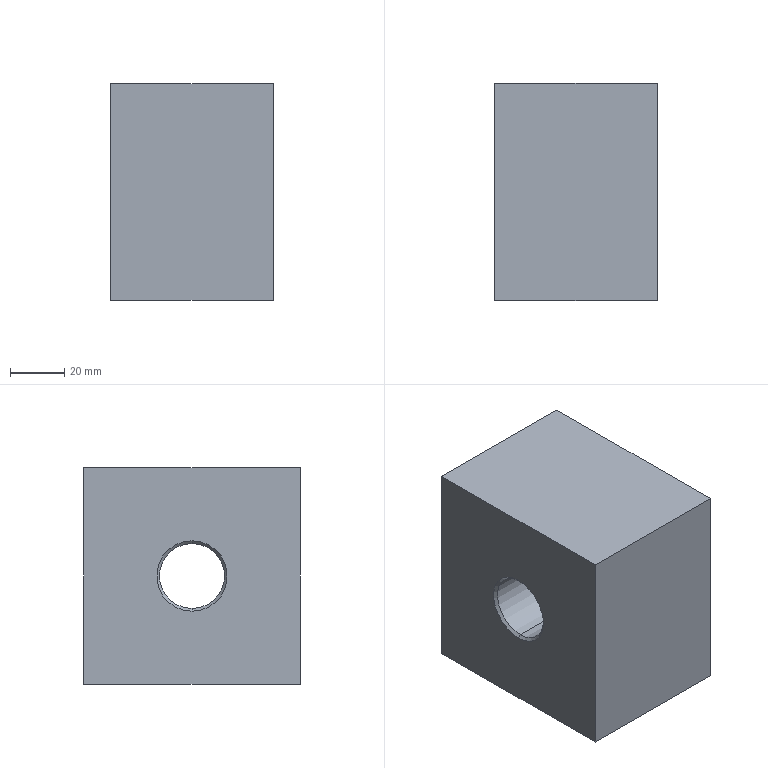Part | SolidWorks | features BaseBody 1 | 1 solid | 28 faces | box 60 x 80 x 80 mm | volume 348755 mm3 | cone 12 | cylinder 10 | plane 6 | commonest cylinder face diameters 8.5 x8 24 x2
STEP:
#1=CARTESIAN_POINT('',(29.,0.,12.));
#2=VERTEX_POINT('',#1);
#3=CARTESIAN_POINT('',(29.,0.,-12.));
#4=VERTEX_POINT('',#3);
#5=CARTESIAN_POINT('',(29.,0.,0.));
#6=DIRECTION('',(1.,0.,0.));
#7=DIRECTION('',(0.,0.,-1.));
#8=AXIS2_PLACEMENT_3D('',#5,#6,#7);
#9=CIRCLE('',#8,12.);
#10=EDGE_CURVE('',#2,#4,#9,.T.);
#11=ORIENTED_EDGE('',*,*,#10,.F.);
#12=CARTESIAN_POINT('',(30.,0.,13.));
#13=VERTEX_POINT('',#12);
#14=CARTESIAN_POINT('',(29.,0.,12.));
#15=DIRECTION('',(0.7071,0.,0.7071));
#16=VECTOR('',#15,1000.);
#17=LINE('',#14,#16);
#18=EDGE_CURVE('',#2,#13,#17,.T.);
#19=ORIENTED_EDGE('',*,*,#18,.T.);
#20=CARTESIAN_POINT('',(30.,0.,-13.));
#21=VERTEX_POINT('',#20);
#22=CARTESIAN_POINT('',(30.,0.,0.));
#23=DIRECTION('',(-1.,0.,0.));
#24=DIRECTION('',(0.,0.,-1.));
#25=AXIS2_PLACEMENT_3D('',#22,#23,#24);
#26=CIRCLE('',#25,13.);
#27=EDGE_CURVE('',#21,#13,#26,.T.);
#28=ORIENTED_EDGE('',*,*,#27,.F.);
#29=CARTESIAN_POINT('',(29.,0.,-12.));
#30=DIRECTION('',(0.7071,0.,-0.7071));
#31=VECTOR('',#30,1000.);
#32=LINE('',#29,#31);
#33=EDGE_CURVE('',#4,#21,#32,.T.);
#34=ORIENTED_EDGE('',*,*,#33,.F.);
#35=EDGE_LOOP('',(#11,#19,#28,#34));
#36=FACE_OUTER_BOUND('',#35,.T.);
#37=CARTESIAN_POINT('',(29.,0.,0.));
#38=DIRECTION('',(1.,0.,0.));
#39=DIRECTION('',(0.,0.,-1.));
#40=AXIS2_PLACEMENT_3D('',#37,#38,#39);
#41=CONICAL_SURFACE('',#40,12.,0.7854);
#42=ADVANCED_FACE('',(#36),#41,.F.);
#43=CARTESIAN_POINT('',(-29.,0.,-12.));
#44=VERTEX_POINT('',#43);
#45=CARTESIAN_POINT('',(-29.,0.,12.));
#46=VERTEX_POINT('',#45);
#47=CARTESIAN_POINT('',(-29.,0.,0.));
#48=DIRECTION('',(-1.,0.,0.));
#49=DIRECTION('',(0.,0.,-1.));
#50=AXIS2_PLACEMENT_3D('',#47,#48,#49);
#51=CIRCLE('',#50,12.);
#52=EDGE_CURVE('',#44,#46,#51,.T.);
#53=ORIENTED_EDGE('',*,*,#52,.F.);
#54=CARTESIAN_POINT('',(-30.,0.,-13.));
#55=VERTEX_POINT('',#54);
#56=CARTESIAN_POINT('',(-30.,0.,-13.));
#57=DIRECTION('',(-0.7071,0.,-0.7071));
#58=VECTOR('',#57,1000.);
#59=LINE('',#56,#58);
#60=EDGE_CURVE('',#44,#55,#59,.T.);
#61=ORIENTED_EDGE('',*,*,#60,.T.);
#62=CARTESIAN_POINT('',(-30.,0.,13.));
#63=VERTEX_POINT('',#62);
#64=CARTESIAN_POINT('',(-30.,0.,0.));
#65=DIRECTION('',(1.,0.,0.));
#66=DIRECTION('',(0.,0.,-1.));
#67=AXIS2_PLACEMENT_3D('',#64,#65,#66);
#68=CIRCLE('',#67,13.);
#69=EDGE_CURVE('',#63,#55,#68,.T.);
#70=ORIENTED_EDGE('',*,*,#69,.F.);
#71=CARTESIAN_POINT('',(-30.,0.,13.));
#72=DIRECTION('',(-0.7071,0.,0.7071));
#73=VECTOR('',#72,1000.);
#74=LINE('',#71,#73);
#75=EDGE_CURVE('',#46,#63,#74,.T.);
#76=ORIENTED_EDGE('',*,*,#75,.F.);
#77=EDGE_LOOP('',(#53,#61,#70,#76));
#78=FACE_OUTER_BOUND('',#77,.T.);
#79=CARTESIAN_POINT('',(-30.,0.,0.));
#80=DIRECTION('',(-1.,0.,0.));
#81=DIRECTION('',(0.,0.,1.));
#82=AXIS2_PLACEMENT_3D('',#79,#80,#81);
#83=CONICAL_SURFACE('',#82,13.,0.7854);
#84=ADVANCED_FACE('',(#78),#83,.F.);
#85=CARTESIAN_POINT('',(-15.,5.5,20.75));
#86=VERTEX_POINT('',#85);
#87=CARTESIAN_POINT('',(-15.,5.5,29.25));
#88=VERTEX_POINT('',#87);
#89=CARTESIAN_POINT('',(-15.,5.5,25.));
#90=DIRECTION('',(0.,1.,0.));
#91=DIRECTION('',(0.,0.,1.));
#92=AXIS2_PLACEMENT_3D('',#89,#90,#91);
#93=CIRCLE('',#92,4.25);
#94=EDGE_CURVE('',#86,#88,#93,.T.);
#95=ORIENTED_EDGE('',*,*,#94,.F.);
#96=CARTESIAN_POINT('',(-15.,40.,20.75));
#97=VERTEX_POINT('',#96);
#98=CARTESIAN_POINT('',(-15.,40.,20.75));
#99=DIRECTION('',(0.,1.,0.));
#100=VECTOR('',#99,1000.);
#101=LINE('',#98,#100);
#102=EDGE_CURVE('',#86,#97,#101,.T.);
#103=ORIENTED_EDGE('',*,*,#102,.T.);
#104=CARTESIAN_POINT('',(-15.,40.,29.25));
#105=VERTEX_POINT('',#104);
#106=CARTESIAN_POINT('',(-15.,40.,25.));
#107=DIRECTION('',(0.,1.,0.));
#108=DIRECTION('',(0.,0.,1.));
#109=AXIS2_PLACEMENT_3D('',#106,#107,#108);
#110=CIRCLE('',#109,4.25);
#111=EDGE_CURVE('',#97,#105,#110,.T.);
#112=ORIENTED_EDGE('',*,*,#111,.T.);
#113=CARTESIAN_POINT('',(-15.,40.,29.25));
#114=DIRECTION('',(0.,1.,0.));
#115=VECTOR('',#114,1000.);
#116=LINE('',#113,#115);
#117=EDGE_CURVE('',#88,#105,#116,.T.);
#118=ORIENTED_EDGE('',*,*,#117,.F.);
#119=EDGE_LOOP('',(#95,#103,#112,#118));
#120=FACE_OUTER_BOUND('',#119,.T.);
#121=CARTESIAN_POINT('',(-15.,40.,25.));
#122=DIRECTION('',(0.,1.,0.));
#123=DIRECTION('',(0.,0.,1.));
#124=AXIS2_PLACEMENT_3D('',#121,#122,#123);
#125=CYLINDRICAL_SURFACE('',#124,4.25);
#126=ADVANCED_FACE('',(#120),#125,.F.);
#127=CARTESIAN_POINT('',(-15.,2.946,25.));
#128=VERTEX_POINT('',#127);
#129=CARTESIAN_POINT('',(-15.,5.5,29.25));
#130=DIRECTION('',(0.,0.515,0.8572));
#131=VECTOR('',#130,1000.);
#132=LINE('',#129,#131);
#133=EDGE_CURVE('',#128,#88,#132,.T.);
#134=ORIENTED_EDGE('',*,*,#133,.F.);
#135=CARTESIAN_POINT('',(-15.,5.5,20.75));
#136=DIRECTION('',(0.,0.515,-0.8572));
#137=VECTOR('',#136,1000.);
#138=LINE('',#135,#137);
#139=EDGE_CURVE('',#128,#86,#138,.T.);
#140=ORIENTED_EDGE('',*,*,#139,.T.);
#141=ORIENTED_EDGE('',*,*,#94,.T.);
#142=EDGE_LOOP('',(#134,#140,#141));
#143=FACE_OUTER_BOUND('',#142,.T.);
#144=CARTESIAN_POINT('',(-15.,5.5,25.));
#145=DIRECTION('',(0.,1.,0.));
#146=DIRECTION('',(0.,0.,1.));
#147=AXIS2_PLACEMENT_3D('',#144,#145,#146);
#148=CONICAL_SURFACE('',#147,4.25,1.03);
#149=ADVANCED_FACE('',(#143),#148,.F.);
#150=CARTESIAN_POINT('',(15.,5.5,20.75));
#151=VERTEX_POINT('',#150);
#152=CARTESIAN_POINT('',(15.,5.5,29.25));
#153=VERTEX_POINT('',#152);
#154=CARTESIAN_POINT('',(15.,5.5,25.));
#155=DIRECTION('',(0.,1.,0.));
#156=DIRECTION('',(0.,0.,1.));
#157=AXIS2_PLACEMENT_3D('',#154,#155,#156);
#158=CIRCLE('',#157,4.25);
#159=EDGE_CURVE('',#151,#153,#158,.T.);
#160=ORIENTED_EDGE('',*,*,#159,.F.);
#161=CARTESIAN_POINT('',(15.,40.,20.75));
#162=VERTEX_POINT('',#161);
#163=CARTESIAN_POINT('',(15.,40.,20.75));
#164=DIRECTION('',(0.,1.,0.));
#165=VECTOR('',#164,1000.);
#166=LINE('',#163,#165);
#167=EDGE_CURVE('',#151,#162,#166,.T.);
#168=ORIENTED_EDGE('',*,*,#167,.T.);
#169=CARTESIAN_POINT('',(15.,40.,29.25));
#170=VERTEX_POINT('',#169);
#171=CARTESIAN_POINT('',(15.,40.,25.));
#172=DIRECTION('',(0.,1.,0.));
#173=DIRECTION('',(0.,0.,1.));
#174=AXIS2_PLACEMENT_3D('',#171,#172,#173);
#175=CIRCLE('',#174,4.25);
#176=EDGE_CURVE('',#162,#170,#175,.T.);
#177=ORIENTED_EDGE('',*,*,#176,.T.);
#178=CARTESIAN_POINT('',(15.,40.,29.25));
#179=DIRECTION('',(0.,1.,0.));
#180=VECTOR('',#179,1000.);
#181=LINE('',#178,#180);
#182=EDGE_CURVE('',#153,#170,#181,.T.);
#183=ORIENTED_EDGE('',*,*,#182,.F.);
#184=EDGE_LOOP('',(#160,#168,#177,#183));
#185=FACE_OUTER_BOUND('',#184,.T.);
#186=CARTESIAN_POINT('',(15.,40.,25.));
#187=DIRECTION('',(0.,1.,0.));
#188=DIRECTION('',(0.,0.,1.));
#189=AXIS2_PLACEMENT_3D('',#186,#187,#188);
#190=CYLINDRICAL_SURFACE('',#189,4.25);
#191=ADVANCED_FACE('',(#185),#190,.F.);
#192=CARTESIAN_POINT('',(15.,2.946,25.));
#193=VERTEX_POINT('',#192);
#194=CARTESIAN_POINT('',(15.,5.5,29.25));
#195=DIRECTION('',(0.,0.515,0.8572));
#196=VECTOR('',#195,1000.);
#197=LINE('',#194,#196);
#198=EDGE_CURVE('',#193,#153,#197,.T.);
#199=ORIENTED_EDGE('',*,*,#198,.F.);
#200=CARTESIAN_POINT('',(15.,5.5,20.75));
#201=DIRECTION('',(0.,0.515,-0.8572));
#202=VECTOR('',#201,1000.);
#203=LINE('',#200,#202);
#204=EDGE_CURVE('',#193,#151,#203,.T.);
#205=ORIENTED_EDGE('',*,*,#204,.T.);
#206=ORIENTED_EDGE('',*,*,#159,.T.);
#207=EDGE_LOOP('',(#199,#205,#206));
#208=FACE_OUTER_BOUND('',#207,.T.);
#209=CARTESIAN_POINT('',(15.,5.5,25.));
#210=DIRECTION('',(0.,1.,0.));
#211=DIRECTION('',(0.,0.,1.));
#212=AXIS2_PLACEMENT_3D('',#209,#210,#211);
#213=CONICAL_SURFACE('',#212,4.25,1.03);
#214=ADVANCED_FACE('',(#208),#213,.F.);
#215=CARTESIAN_POINT('',(15.,5.5,-29.25));
#216=VERTEX_POINT('',#215);
#217=CARTESIAN_POINT('',(15.,5.5,-20.75));
#218=VERTEX_POINT('',#217);
#219=CARTESIAN_POINT('',(15.,5.5,-25.));
#220=DIRECTION('',(0.,1.,0.));
#221=DIRECTION('',(0.,0.,1.));
#222=AXIS2_PLACEMENT_3D('',#219,#220,#221);
#223=CIRCLE('',#222,4.25);
#224=EDGE_CURVE('',#216,#218,#223,.T.);
#225=ORIENTED_EDGE('',*,*,#224,.F.);
#226=CARTESIAN_POINT('',(15.,40.,-29.25));
#227=VERTEX_POINT('',#226);
#228=CARTESIAN_POINT('',(15.,40.,-29.25));
#229=DIRECTION('',(0.,1.,0.));
#230=VECTOR('',#229,1000.);
#231=LINE('',#228,#230);
#232=EDGE_CURVE('',#216,#227,#231,.T.);
#233=ORIENTED_EDGE('',*,*,#232,.T.);
#234=CARTESIAN_POINT('',(15.,40.,-20.75));
#235=VERTEX_POINT('',#234);
#236=CARTESIAN_POINT('',(15.,40.,-25.));
#237=DIRECTION('',(0.,1.,0.));
#238=DIRECTION('',(0.,0.,1.));
#239=AXIS2_PLACEMENT_3D('',#236,#237,#238);
#240=CIRCLE('',#239,4.25);
#241=EDGE_CURVE('',#227,#235,#240,.T.);
#242=ORIENTED_EDGE('',*,*,#241,.T.);
#243=CARTESIAN_POINT('',(15.,40.,-20.75));
#244=DIRECTION('',(0.,1.,0.));
#245=VECTOR('',#244,1000.);
#246=LINE('',#243,#245);
#247=EDGE_CURVE('',#218,#235,#246,.T.);
#248=ORIENTED_EDGE('',*,*,#247,.F.);
#249=EDGE_LOOP('',(#225,#233,#242,#248));
#250=FACE_OUTER_BOUND('',#249,.T.);
#251=CARTESIAN_POINT('',(15.,40.,-25.));
#252=DIRECTION('',(0.,1.,0.));
#253=DIRECTION('',(0.,0.,1.));
#254=AXIS2_PLACEMENT_3D('',#251,#252,#253);
#255=CYLINDRICAL_SURFACE('',#254,4.25);
#256=ADVANCED_FACE('',(#250),#255,.F.);
#257=CARTESIAN_POINT('',(15.,2.946,-25.));
#258=VERTEX_POINT('',#257);
#259=CARTESIAN_POINT('',(15.,5.5,-20.75));
#260=DIRECTION('',(0.,0.515,0.8572));
#261=VECTOR('',#260,1000.);
#262=LINE('',#259,#261);
#263=EDGE_CURVE('',#258,#218,#262,.T.);
#264=ORIENTED_EDGE('',*,*,#263,.F.);
#265=CARTESIAN_POINT('',(15.,5.5,-29.25));
#266=DIRECTION('',(0.,0.515,-0.8572));
#267=VECTOR('',#266,1000.);
#268=LINE('',#265,#267);
#269=EDGE_CURVE('',#258,#216,#268,.T.);
#270=ORIENTED_EDGE('',*,*,#269,.T.);
#271=ORIENTED_EDGE('',*,*,#224,.T.);
#272=EDGE_LOOP('',(#264,#270,#271));
#273=FACE_OUTER_BOUND('',#272,.T.);
#274=CARTESIAN_POINT('',(15.,5.5,-25.));
#275=DIRECTION('',(0.,1.,0.));
#276=DIRECTION('',(0.,0.,1.));
#277=AXIS2_PLACEMENT_3D('',#274,#275,#276);
#278=CONICAL_SURFACE('',#277,4.25,1.03);
#279=ADVANCED_FACE('',(#273),#278,.F.);
#280=CARTESIAN_POINT('',(-15.,5.5,-29.25));
#281=VERTEX_POINT('',#280);
#282=CARTESIAN_POINT('',(-15.,5.5,-20.75));
#283=VERTEX_POINT('',#282);
#284=CARTESIAN_POINT('',(-15.,5.5,-25.));
#285=DIRECTION('',(0.,1.,0.));
#286=DIRECTION('',(0.,0.,1.));
#287=AXIS2_PLACEMENT_3D('',#284,#285,#286);
#288=CIRCLE('',#287,4.25);
#289=EDGE_CURVE('',#281,#283,#288,.T.);
#290=ORIENTED_EDGE('',*,*,#289,.F.);
#291=CARTESIAN_POINT('',(-15.,40.,-29.25));
#292=VERTEX_POINT('',#291);
#293=CARTESIAN_POINT('',(-15.,40.,-29.25));
#294=DIRECTION('',(0.,1.,0.));
#295=VECTOR('',#294,1000.);
#296=LINE('',#293,#295);
#297=EDGE_CURVE('',#281,#292,#296,.T.);
#298=ORIENTED_EDGE('',*,*,#297,.T.);
#299=CARTESIAN_POINT('',(-15.,40.,-20.75));
#300=VERTEX_POINT('',#299);
#301=CARTESIAN_POINT('',(-15.,40.,-25.));
#302=DIRECTION('',(0.,1.,0.));
#303=DIRECTION('',(0.,0.,1.));
#304=AXIS2_PLACEMENT_3D('',#301,#302,#303);
#305=CIRCLE('',#304,4.25);
#306=EDGE_CURVE('',#292,#300,#305,.T.);
#307=ORIENTED_EDGE('',*,*,#306,.T.);
#308=CARTESIAN_POINT('',(-15.,40.,-20.75));
#309=DIRECTION('',(0.,1.,0.));
#310=VECTOR('',#309,1000.);
#311=LINE('',#308,#310);
#312=EDGE_CURVE('',#283,#300,#311,.T.);
#313=ORIENTED_EDGE('',*,*,#312,.F.);
#314=EDGE_LOOP('',(#290,#298,#307,#313));
#315=FACE_OUTER_BOUND('',#314,.T.);
#316=CARTESIAN_POINT('',(-15.,40.,-25.));
#317=DIRECTION('',(0.,1.,0.));
#318=DIRECTION('',(0.,0.,1.));
#319=AXIS2_PLACEMENT_3D('',#316,#317,#318);
#320=CYLINDRICAL_SURFACE('',#319,4.25);
#321=ADVANCED_FACE('',(#315),#320,.F.);
#322=CARTESIAN_POINT('',(-15.,2.946,-25.));
#323=VERTEX_POINT('',#322);
#324=CARTESIAN_POINT('',(-15.,5.5,-20.75));
#325=DIRECTION('',(0.,0.515,0.8572));
#326=VECTOR('',#325,1000.);
#327=LINE('',#324,#326);
#328=EDGE_CURVE('',#323,#283,#327,.T.);
#329=ORIENTED_EDGE('',*,*,#328,.F.);
#330=CARTESIAN_POINT('',(-15.,5.5,-29.25));
#331=DIRECTION('',(0.,0.515,-0.8572));
#332=VECTOR('',#331,1000.);
#333=LINE('',#330,#332);
#334=EDGE_CURVE('',#323,#281,#333,.T.);
#335=ORIENTED_EDGE('',*,*,#334,.T.);
#336=ORIENTED_EDGE('',*,*,#289,.T.);
#337=EDGE_LOOP('',(#329,#335,#336));
#338=FACE_OUTER_BOUND('',#337,.T.);
#339=CARTESIAN_POINT('',(-15.,5.5,-25.));
#340=DIRECTION('',(0.,1.,0.));
#341=DIRECTION('',(0.,0.,1.));
#342=AXIS2_PLACEMENT_3D('',#339,#340,#341);
#343=CONICAL_SURFACE('',#342,4.25,1.03);
#344=ADVANCED_FACE('',(#338),#343,.F.);
#345=ORIENTED_EDGE('',*,*,#52,.T.);
#346=CARTESIAN_POINT('',(30.,0.,12.));
#347=DIRECTION('',(1.,0.,0.));
#348=VECTOR('',#347,1000.);
#349=LINE('',#346,#348);
#350=EDGE_CURVE('',#46,#2,#349,.T.);
#351=ORIENTED_EDGE('',*,*,#350,.T.);
#352=ORIENTED_EDGE('',*,*,#10,.T.);
#353=CARTESIAN_POINT('',(30.,0.,-12.));
#354=DIRECTION('',(1.,0.,0.));
#355=VECTOR('',#354,1000.);
#356=LINE('',#353,#355);
#357=EDGE_CURVE('',#44,#4,#356,.T.);
#358=ORIENTED_EDGE('',*,*,#357,.F.);
#359=EDGE_LOOP('',(#345,#351,#352,#358));
#360=FACE_OUTER_BOUND('',#359,.T.);
#361=CARTESIAN_POINT('',(30.,0.,0.));
#362=DIRECTION('',(1.,0.,0.));
#363=DIRECTION('',(0.,0.,-1.));
#364=AXIS2_PLACEMENT_3D('',#361,#362,#363);
#365=CYLINDRICAL_SURFACE('',#364,12.);
#366=ADVANCED_FACE('',(#360),#365,.F.);
#367=CARTESIAN_POINT('',(-30.,-40.,-40.));
#368=VERTEX_POINT('',#367);
#369=CARTESIAN_POINT('',(-30.,40.,-40.));
#370=VERTEX_POINT('',#369);
#371=CARTESIAN_POINT('',(-30.,40.,-40.));
#372=DIRECTION('',(0.,1.,0.));
#373=VECTOR('',#372,1000.);
#374=LINE('',#371,#373);
#375=EDGE_CURVE('',#368,#370,#374,.T.);
#376=ORIENTED_EDGE('',*,*,#375,.T.);
#377=CARTESIAN_POINT('',(30.,40.,-40.));
#378=VERTEX_POINT('',#377);
#379=CARTESIAN_POINT('',(30.,40.,-40.));
#380=DIRECTION('',(-1.,0.,0.));
#381=VECTOR('',#380,1000.);
#382=LINE('',#379,#381);
#383=EDGE_CURVE('',#378,#370,#382,.T.);
#384=ORIENTED_EDGE('',*,*,#383,.F.);
#385=CARTESIAN_POINT('',(30.,-40.,-40.));
#386=VERTEX_POINT('',#385);
#387=CARTESIAN_POINT('',(30.,40.,-40.));
#388=DIRECTION('',(0.,1.,0.));
#389=VECTOR('',#388,1000.);
#390=LINE('',#387,#389);
#391=EDGE_CURVE('',#386,#378,#390,.T.);
#392=ORIENTED_EDGE('',*,*,#391,.F.);
#393=CARTESIAN_POINT('',(30.,-40.,-40.));
#394=DIRECTION('',(-1.,0.,0.));
#395=VECTOR('',#394,1000.);
#396=LINE('',#393,#395);
#397=EDGE_CURVE('',#386,#368,#396,.T.);
#398=ORIENTED_EDGE('',*,*,#397,.T.);
#399=EDGE_LOOP('',(#376,#384,#392,#398));
#400=FACE_OUTER_BOUND('',#399,.T.);
#401=CARTESIAN_POINT('',(30.,40.,-40.));
#402=DIRECTION('',(0.,0.,1.));
#403=DIRECTION('',(0.,-1.,0.));
#404=AXIS2_PLACEMENT_3D('',#401,#402,#403);
#405=PLANE('',#404);
#406=ADVANCED_FACE('',(#400),#405,.F.);
#407=CARTESIAN_POINT('',(-15.,40.,25.));
#408=DIRECTION('',(0.,1.,0.));
#409=DIRECTION('',(0.,0.,1.));
#410=AXIS2_PLACEMENT_3D('',#407,#408,#409);
#411=CIRCLE('',#410,4.25);
#412=EDGE_CURVE('',#105,#97,#411,.T.);
#413=ORIENTED_EDGE('',*,*,#412,.F.);
#414=ORIENTED_EDGE('',*,*,#111,.F.);
#415=EDGE_LOOP('',(#413,#414));
#416=FACE_BOUND('',#415,.T.);
#417=CARTESIAN_POINT('',(15.,40.,25.));
#418=DIRECTION('',(0.,1.,0.));
#419=DIRECTION('',(0.,0.,1.));
#420=AXIS2_PLACEMENT_3D('',#417,#418,#419);
#421=CIRCLE('',#420,4.25);
#422=EDGE_CURVE('',#170,#162,#421,.T.);
#423=ORIENTED_EDGE('',*,*,#422,.F.);
#424=ORIENTED_EDGE('',*,*,#176,.F.);
#425=EDGE_LOOP('',(#423,#424));
#426=FACE_BOUND('',#425,.T.);
#427=CARTESIAN_POINT('',(15.,40.,-25.));
#428=DIRECTION('',(0.,1.,0.));
#429=DIRECTION('',(0.,0.,1.));
#430=AXIS2_PLACEMENT_3D('',#427,#428,#429);
#431=CIRCLE('',#430,4.25);
#432=EDGE_CURVE('',#235,#227,#431,.T.);
#433=ORIENTED_EDGE('',*,*,#432,.F.);
#434=ORIENTED_EDGE('',*,*,#241,.F.);
#435=EDGE_LOOP('',(#433,#434));
#436=FACE_BOUND('',#435,.T.);
#437=CARTESIAN_POINT('',(-15.,40.,-25.));
#438=DIRECTION('',(0.,1.,0.));
#439=DIRECTION('',(0.,0.,1.));
#440=AXIS2_PLACEMENT_3D('',#437,#438,#439);
#441=CIRCLE('',#440,4.25);
#442=EDGE_CURVE('',#300,#292,#441,.T.);
#443=ORIENTED_EDGE('',*,*,#442,.F.);
#444=ORIENTED_EDGE('',*,*,#306,.F.);
#445=EDGE_LOOP('',(#443,#444));
#446=FACE_BOUND('',#445,.T.);
#447=CARTESIAN_POINT('',(-30.,40.,40.));
#448=VERTEX_POINT('',#447);
#449=CARTESIAN_POINT('',(-30.,40.,40.));
#450=DIRECTION('',(0.,0.,1.));
#451=VECTOR('',#450,1000.);
#452=LINE('',#449,#451);
#453=EDGE_CURVE('',#370,#448,#452,.T.);
#454=ORIENTED_EDGE('',*,*,#453,.T.);
#455=CARTESIAN_POINT('',(30.,40.,40.));
#456=VERTEX_POINT('',#455);
#457=CARTESIAN_POINT('',(30.,40.,40.));
#458=DIRECTION('',(-1.,0.,0.));
#459=VECTOR('',#458,1000.);
#460=LINE('',#457,#459);
#461=EDGE_CURVE('',#456,#448,#460,.T.);
#462=ORIENTED_EDGE('',*,*,#461,.F.);
#463=CARTESIAN_POINT('',(30.,40.,40.));
#464=DIRECTION('',(0.,0.,1.));
#465=VECTOR('',#464,1000.);
#466=LINE('',#463,#465);
#467=EDGE_CURVE('',#378,#456,#466,.T.);
#468=ORIENTED_EDGE('',*,*,#467,.F.);
#469=ORIENTED_EDGE('',*,*,#383,.T.);
#470=EDGE_LOOP('',(#454,#462,#468,#469));
#471=FACE_OUTER_BOUND('',#470,.T.);
#472=CARTESIAN_POINT('',(30.,40.,40.));
#473=DIRECTION('',(0.,-1.,0.));
#474=DIRECTION('',(0.,0.,-1.));
#475=AXIS2_PLACEMENT_3D('',#472,#473,#474);
#476=PLANE('',#475);
#477=ADVANCED_FACE('',(#416,#426,#436,#446,#471),#476,.F.);
#478=CARTESIAN_POINT('',(-30.,-40.,40.));
#479=VERTEX_POINT('',#478);
#480=CARTESIAN_POINT('',(-30.,40.,40.));
#481=DIRECTION('',(0.,-1.,0.));
#482=VECTOR('',#481,1000.);
#483=LINE('',#480,#482);
#484=EDGE_CURVE('',#448,#479,#483,.T.);
#485=ORIENTED_EDGE('',*,*,#484,.T.);
#486=CARTESIAN_POINT('',(30.,-40.,40.));
#487=VERTEX_POINT('',#486);
#488=CARTESIAN_POINT('',(30.,-40.,40.));
#489=DIRECTION('',(-1.,0.,0.));
#490=VECTOR('',#489,1000.);
#491=LINE('',#488,#490);
#492=EDGE_CURVE('',#487,#479,#491,.T.);
#493=ORIENTED_EDGE('',*,*,#492,.F.);
#494=CARTESIAN_POINT('',(30.,40.,40.));
#495=DIRECTION('',(0.,-1.,0.));
#496=VECTOR('',#495,1000.);
#497=LINE('',#494,#496);
#498=EDGE_CURVE('',#456,#487,#497,.T.);
#499=ORIENTED_EDGE('',*,*,#498,.F.);
#500=ORIENTED_EDGE('',*,*,#461,.T.);
#501=EDGE_LOOP('',(#485,#493,#499,#500));
#502=FACE_OUTER_BOUND('',#501,.T.);
#503=CARTESIAN_POINT('',(30.,40.,40.));
#504=DIRECTION('',(0.,0.,-1.));
#505=DIRECTION('',(0.,1.,0.));
#506=AXIS2_PLACEMENT_3D('',#503,#504,#505);
#507=PLANE('',#506);
#508=ADVANCED_FACE('',(#502),#507,.F.);
#509=CARTESIAN_POINT('',(-30.,-40.,40.));
#510=DIRECTION('',(0.,0.,-1.));
#511=VECTOR('',#510,1000.);
#512=LINE('',#509,#511);
#513=EDGE_CURVE('',#479,#368,#512,.T.);
#514=ORIENTED_EDGE('',*,*,#513,.T.);
#515=ORIENTED_EDGE('',*,*,#397,.F.);
#516=CARTESIAN_POINT('',(30.,-40.,40.));
#517=DIRECTION('',(0.,0.,-1.));
#518=VECTOR('',#517,1000.);
#519=LINE('',#516,#518);
#520=EDGE_CURVE('',#487,#386,#519,.T.);
#521=ORIENTED_EDGE('',*,*,#520,.F.);
#522=ORIENTED_EDGE('',*,*,#492,.T.);
#523=EDGE_LOOP('',(#514,#515,#521,#522));
#524=FACE_OUTER_BOUND('',#523,.T.);
#525=CARTESIAN_POINT('',(30.,-40.,40.));
#526=DIRECTION('',(0.,1.,0.));
#527=DIRECTION('',(0.,0.,1.));
#528=AXIS2_PLACEMENT_3D('',#525,#526,#527);
#529=PLANE('',#528);
#530=ADVANCED_FACE('',(#524),#529,.F.);
#531=ORIENTED_EDGE('',*,*,#27,.T.);
#532=CARTESIAN_POINT('',(30.,0.,0.));
#533=DIRECTION('',(-1.,0.,0.));
#534=DIRECTION('',(0.,0.,-1.));
#535=AXIS2_PLACEMENT_3D('',#532,#533,#534);
#536=CIRCLE('',#535,13.);
#537=EDGE_CURVE('',#13,#21,#536,.T.);
#538=ORIENTED_EDGE('',*,*,#537,.T.);
#539=EDGE_LOOP('',(#531,#538));
#540=FACE_BOUND('',#539,.T.);
#541=ORIENTED_EDGE('',*,*,#391,.T.);
#542=ORIENTED_EDGE('',*,*,#467,.T.);
#543=ORIENTED_EDGE('',*,*,#498,.T.);
#544=ORIENTED_EDGE('',*,*,#520,.T.);
#545=EDGE_LOOP('',(#541,#542,#543,#544));
#546=FACE_OUTER_BOUND('',#545,.T.);
#547=CARTESIAN_POINT('',(30.,0.,0.));
#548=DIRECTION('',(1.,0.,0.));
#549=DIRECTION('',(0.,0.,-1.));
#550=AXIS2_PLACEMENT_3D('',#547,#548,#549);
#551=PLANE('',#550);
#552=ADVANCED_FACE('',(#540,#546),#551,.T.);
#553=ORIENTED_EDGE('',*,*,#69,.T.);
#554=CARTESIAN_POINT('',(-30.,0.,0.));
#555=DIRECTION('',(1.,0.,0.));
#556=DIRECTION('',(0.,0.,-1.));
#557=AXIS2_PLACEMENT_3D('',#554,#555,#556);
#558=CIRCLE('',#557,13.);
#559=EDGE_CURVE('',#55,#63,#558,.T.);
#560=ORIENTED_EDGE('',*,*,#559,.T.);
#561=EDGE_LOOP('',(#553,#560));
#562=FACE_BOUND('',#561,.T.);
#563=ORIENTED_EDGE('',*,*,#375,.F.);
#564=ORIENTED_EDGE('',*,*,#513,.F.);
#565=ORIENTED_EDGE('',*,*,#484,.F.);
#566=ORIENTED_EDGE('',*,*,#453,.F.);
#567=EDGE_LOOP('',(#563,#564,#565,#566));
#568=FACE_OUTER_BOUND('',#567,.T.);
#569=CARTESIAN_POINT('',(-30.,0.,0.));
#570=DIRECTION('',(1.,0.,0.));
#571=DIRECTION('',(0.,0.,-1.));
#572=AXIS2_PLACEMENT_3D('',#569,#570,#571);
#573=PLANE('',#572);
#574=ADVANCED_FACE('',(#562,#568),#573,.F.);
#575=ORIENTED_EDGE('',*,*,#350,.F.);
#576=CARTESIAN_POINT('',(-29.,0.,0.));
#577=DIRECTION('',(-1.,0.,0.));
#578=DIRECTION('',(0.,0.,-1.));
#579=AXIS2_PLACEMENT_3D('',#576,#577,#578);
#580=CIRCLE('',#579,12.);
#581=EDGE_CURVE('',#46,#44,#580,.T.);
#582=ORIENTED_EDGE('',*,*,#581,.T.);
#583=ORIENTED_EDGE('',*,*,#357,.T.);
#584=CARTESIAN_POINT('',(29.,0.,0.));
#585=DIRECTION('',(1.,0.,0.));
#586=DIRECTION('',(0.,0.,-1.));
#587=AXIS2_PLACEMENT_3D('',#584,#585,#586);
#588=CIRCLE('',#587,12.);
#589=EDGE_CURVE('',#4,#2,#588,.T.);
#590=ORIENTED_EDGE('',*,*,#589,.T.);
#591=EDGE_LOOP('',(#575,#582,#583,#590));
#592=FACE_OUTER_BOUND('',#591,.T.);
#593=CARTESIAN_POINT('',(30.,0.,0.));
#594=DIRECTION('',(1.,0.,0.));
#595=DIRECTION('',(0.,0.,-1.));
#596=AXIS2_PLACEMENT_3D('',#593,#594,#595);
#597=CYLINDRICAL_SURFACE('',#596,12.);
#598=ADVANCED_FACE('',(#592),#597,.F.);
#599=ORIENTED_EDGE('',*,*,#334,.F.);
#600=ORIENTED_EDGE('',*,*,#328,.T.);
#601=CARTESIAN_POINT('',(-15.,5.5,-25.));
#602=DIRECTION('',(0.,1.,0.));
#603=DIRECTION('',(0.,0.,1.));
#604=AXIS2_PLACEMENT_3D('',#601,#602,#603);
#605=CIRCLE('',#604,4.25);
#606=EDGE_CURVE('',#283,#281,#605,.T.);
#607=ORIENTED_EDGE('',*,*,#606,.T.);
#608=EDGE_LOOP('',(#599,#600,#607));
#609=FACE_OUTER_BOUND('',#608,.T.);
#610=CARTESIAN_POINT('',(-15.,5.5,-25.));
#611=DIRECTION('',(0.,1.,0.));
#612=DIRECTION('',(0.,0.,1.));
#613=AXIS2_PLACEMENT_3D('',#610,#611,#612);
#614=CONICAL_SURFACE('',#613,4.25,1.03);
#615=ADVANCED_FACE('',(#609),#614,.F.);
#616=ORIENTED_EDGE('',*,*,#297,.F.);
#617=ORIENTED_EDGE('',*,*,#606,.F.);
#618=ORIENTED_EDGE('',*,*,#312,.T.);
#619=ORIENTED_EDGE('',*,*,#442,.T.);
#620=EDGE_LOOP('',(#616,#617,#618,#619));
#621=FACE_OUTER_BOUND('',#620,.T.);
#622=CARTESIAN_POINT('',(-15.,40.,-25.));
#623=DIRECTION('',(0.,1.,0.));
#624=DIRECTION('',(0.,0.,1.));
#625=AXIS2_PLACEMENT_3D('',#622,#623,#624);
#626=CYLINDRICAL_SURFACE('',#625,4.25);
#627=ADVANCED_FACE('',(#621),#626,.F.);
#628=ORIENTED_EDGE('',*,*,#269,.F.);
#629=ORIENTED_EDGE('',*,*,#263,.T.);
#630=CARTESIAN_POINT('',(15.,5.5,-25.));
#631=DIRECTION('',(0.,1.,0.));
#632=DIRECTION('',(0.,0.,1.));
#633=AXIS2_PLACEMENT_3D('',#630,#631,#632);
#634=CIRCLE('',#633,4.25);
#635=EDGE_CURVE('',#218,#216,#634,.T.);
#636=ORIENTED_EDGE('',*,*,#635,.T.);
#637=EDGE_LOOP('',(#628,#629,#636));
#638=FACE_OUTER_BOUND('',#637,.T.);
#639=CARTESIAN_POINT('',(15.,5.5,-25.));
#640=DIRECTION('',(0.,1.,0.));
#641=DIRECTION('',(0.,0.,1.));
#642=AXIS2_PLACEMENT_3D('',#639,#640,#641);
#643=CONICAL_SURFACE('',#642,4.25,1.03);
#644=ADVANCED_FACE('',(#638),#643,.F.);
#645=ORIENTED_EDGE('',*,*,#232,.F.);
#646=ORIENTED_EDGE('',*,*,#635,.F.);
#647=ORIENTED_EDGE('',*,*,#247,.T.);
#648=ORIENTED_EDGE('',*,*,#432,.T.);
#649=EDGE_LOOP('',(#645,#646,#647,#648));
#650=FACE_OUTER_BOUND('',#649,.T.);
#651=CARTESIAN_POINT('',(15.,40.,-25.));
#652=DIRECTION('',(0.,1.,0.));
#653=DIRECTION('',(0.,0.,1.));
#654=AXIS2_PLACEMENT_3D('',#651,#652,#653);
#655=CYLINDRICAL_SURFACE('',#654,4.25);
#656=ADVANCED_FACE('',(#650),#655,.F.);
#657=ORIENTED_EDGE('',*,*,#204,.F.);
#658=ORIENTED_EDGE('',*,*,#198,.T.);
#659=CARTESIAN_POINT('',(15.,5.5,25.));
#660=DIRECTION('',(0.,1.,0.));
#661=DIRECTION('',(0.,0.,1.));
#662=AXIS2_PLACEMENT_3D('',#659,#660,#661);
#663=CIRCLE('',#662,4.25);
#664=EDGE_CURVE('',#153,#151,#663,.T.);
#665=ORIENTED_EDGE('',*,*,#664,.T.);
#666=EDGE_LOOP('',(#657,#658,#665));
#667=FACE_OUTER_BOUND('',#666,.T.);
#668=CARTESIAN_POINT('',(15.,5.5,25.));
#669=DIRECTION('',(0.,1.,0.));
#670=DIRECTION('',(0.,0.,1.));
#671=AXIS2_PLACEMENT_3D('',#668,#669,#670);
#672=CONICAL_SURFACE('',#671,4.25,1.03);
#673=ADVANCED_FACE('',(#667),#672,.F.);
#674=ORIENTED_EDGE('',*,*,#167,.F.);
#675=ORIENTED_EDGE('',*,*,#664,.F.);
#676=ORIENTED_EDGE('',*,*,#182,.T.);
#677=ORIENTED_EDGE('',*,*,#422,.T.);
#678=EDGE_LOOP('',(#674,#675,#676,#677));
#679=FACE_OUTER_BOUND('',#678,.T.);
#680=CARTESIAN_POINT('',(15.,40.,25.));
#681=DIRECTION('',(0.,1.,0.));
#682=DIRECTION('',(0.,0.,1.));
#683=AXIS2_PLACEMENT_3D('',#680,#681,#682);
#684=CYLINDRICAL_SURFACE('',#683,4.25);
#685=ADVANCED_FACE('',(#679),#684,.F.);
#686=ORIENTED_EDGE('',*,*,#139,.F.);
#687=ORIENTED_EDGE('',*,*,#133,.T.);
#688=CARTESIAN_POINT('',(-15.,5.5,25.));
#689=DIRECTION('',(0.,1.,0.));
#690=DIRECTION('',(0.,0.,1.));
#691=AXIS2_PLACEMENT_3D('',#688,#689,#690);
#692=CIRCLE('',#691,4.25);
#693=EDGE_CURVE('',#88,#86,#692,.T.);
#694=ORIENTED_EDGE('',*,*,#693,.T.);
#695=EDGE_LOOP('',(#686,#687,#694));
#696=FACE_OUTER_BOUND('',#695,.T.);
#697=CARTESIAN_POINT('',(-15.,5.5,25.));
#698=DIRECTION('',(0.,1.,0.));
#699=DIRECTION('',(0.,0.,1.));
#700=AXIS2_PLACEMENT_3D('',#697,#698,#699);
#701=CONICAL_SURFACE('',#700,4.25,1.03);
#702=ADVANCED_FACE('',(#696),#701,.F.);
#703=ORIENTED_EDGE('',*,*,#102,.F.);
#704=ORIENTED_EDGE('',*,*,#693,.F.);
#705=ORIENTED_EDGE('',*,*,#117,.T.);
#706=ORIENTED_EDGE('',*,*,#412,.T.);
#707=EDGE_LOOP('',(#703,#704,#705,#706));
#708=FACE_OUTER_BOUND('',#707,.T.);
#709=CARTESIAN_POINT('',(-15.,40.,25.));
#710=DIRECTION('',(0.,1.,0.));
#711=DIRECTION('',(0.,0.,1.));
#712=AXIS2_PLACEMENT_3D('',#709,#710,#711);
#713=CYLINDRICAL_SURFACE('',#712,4.25);
#714=ADVANCED_FACE('',(#708),#713,.F.);
#715=ORIENTED_EDGE('',*,*,#60,.F.);
#716=ORIENTED_EDGE('',*,*,#581,.F.);
#717=ORIENTED_EDGE('',*,*,#75,.T.);
#718=ORIENTED_EDGE('',*,*,#559,.F.);
#719=EDGE_LOOP('',(#715,#716,#717,#718));
#720=FACE_OUTER_BOUND('',#719,.T.);
#721=CARTESIAN_POINT('',(-30.,0.,0.));
#722=DIRECTION('',(-1.,0.,0.));
#723=DIRECTION('',(0.,0.,1.));
#724=AXIS2_PLACEMENT_3D('',#721,#722,#723);
#725=CONICAL_SURFACE('',#724,13.,0.7854);
#726=ADVANCED_FACE('',(#720),#725,.F.);
#727=ORIENTED_EDGE('',*,*,#18,.F.);
#728=ORIENTED_EDGE('',*,*,#589,.F.);
#729=ORIENTED_EDGE('',*,*,#33,.T.);
#730=ORIENTED_EDGE('',*,*,#537,.F.);
#731=EDGE_LOOP('',(#727,#728,#729,#730));
#732=FACE_OUTER_BOUND('',#731,.T.);
#733=CARTESIAN_POINT('',(29.,0.,0.));
#734=DIRECTION('',(1.,0.,0.));
#735=DIRECTION('',(0.,0.,-1.));
#736=AXIS2_PLACEMENT_3D('',#733,#734,#735);
#737=CONICAL_SURFACE('',#736,12.,0.7854);
#738=ADVANCED_FACE('',(#732),#737,.F.);
#739=CLOSED_SHELL('',(#42,#84,#126,#149,#191,#214,#256,#279,#321,#344,#366,#406,#477,#508,#530,#552,#574,#598,#615,#627,#644,#656,#673,#685,#702,#714,#726,#738));
#740=MANIFOLD_SOLID_BREP('',#739);
#741=CARTESIAN_POINT('',(0.,0.,0.));
#742=DIRECTION('',(0.,0.,1.));
#743=DIRECTION('',(1.,0.,0.));
#744=AXIS2_PLACEMENT_3D('',#741,#742,#743);
#745=(LENGTH_UNIT()NAMED_UNIT(*)SI_UNIT(.MILLI.,.METRE.));
#746=UNCERTAINTY_MEASURE_WITH_UNIT(LENGTH_MEASURE(0.00001),#745,'','');
#747=(NAMED_UNIT(*)PLANE_ANGLE_UNIT()SI_UNIT($,.RADIAN.));
#748=(NAMED_UNIT(*)SI_UNIT($,.STERADIAN.)SOLID_ANGLE_UNIT());
#749=(GEOMETRIC_REPRESENTATION_CONTEXT(3)GLOBAL_UNCERTAINTY_ASSIGNED_CONTEXT((#746))GLOBAL_UNIT_ASSIGNED_CONTEXT((#745,#747,#748))REPRESENTATION_CONTEXT('',''));
#750=ADVANCED_BREP_SHAPE_REPRESENTATION('',(#740,#744),#749);